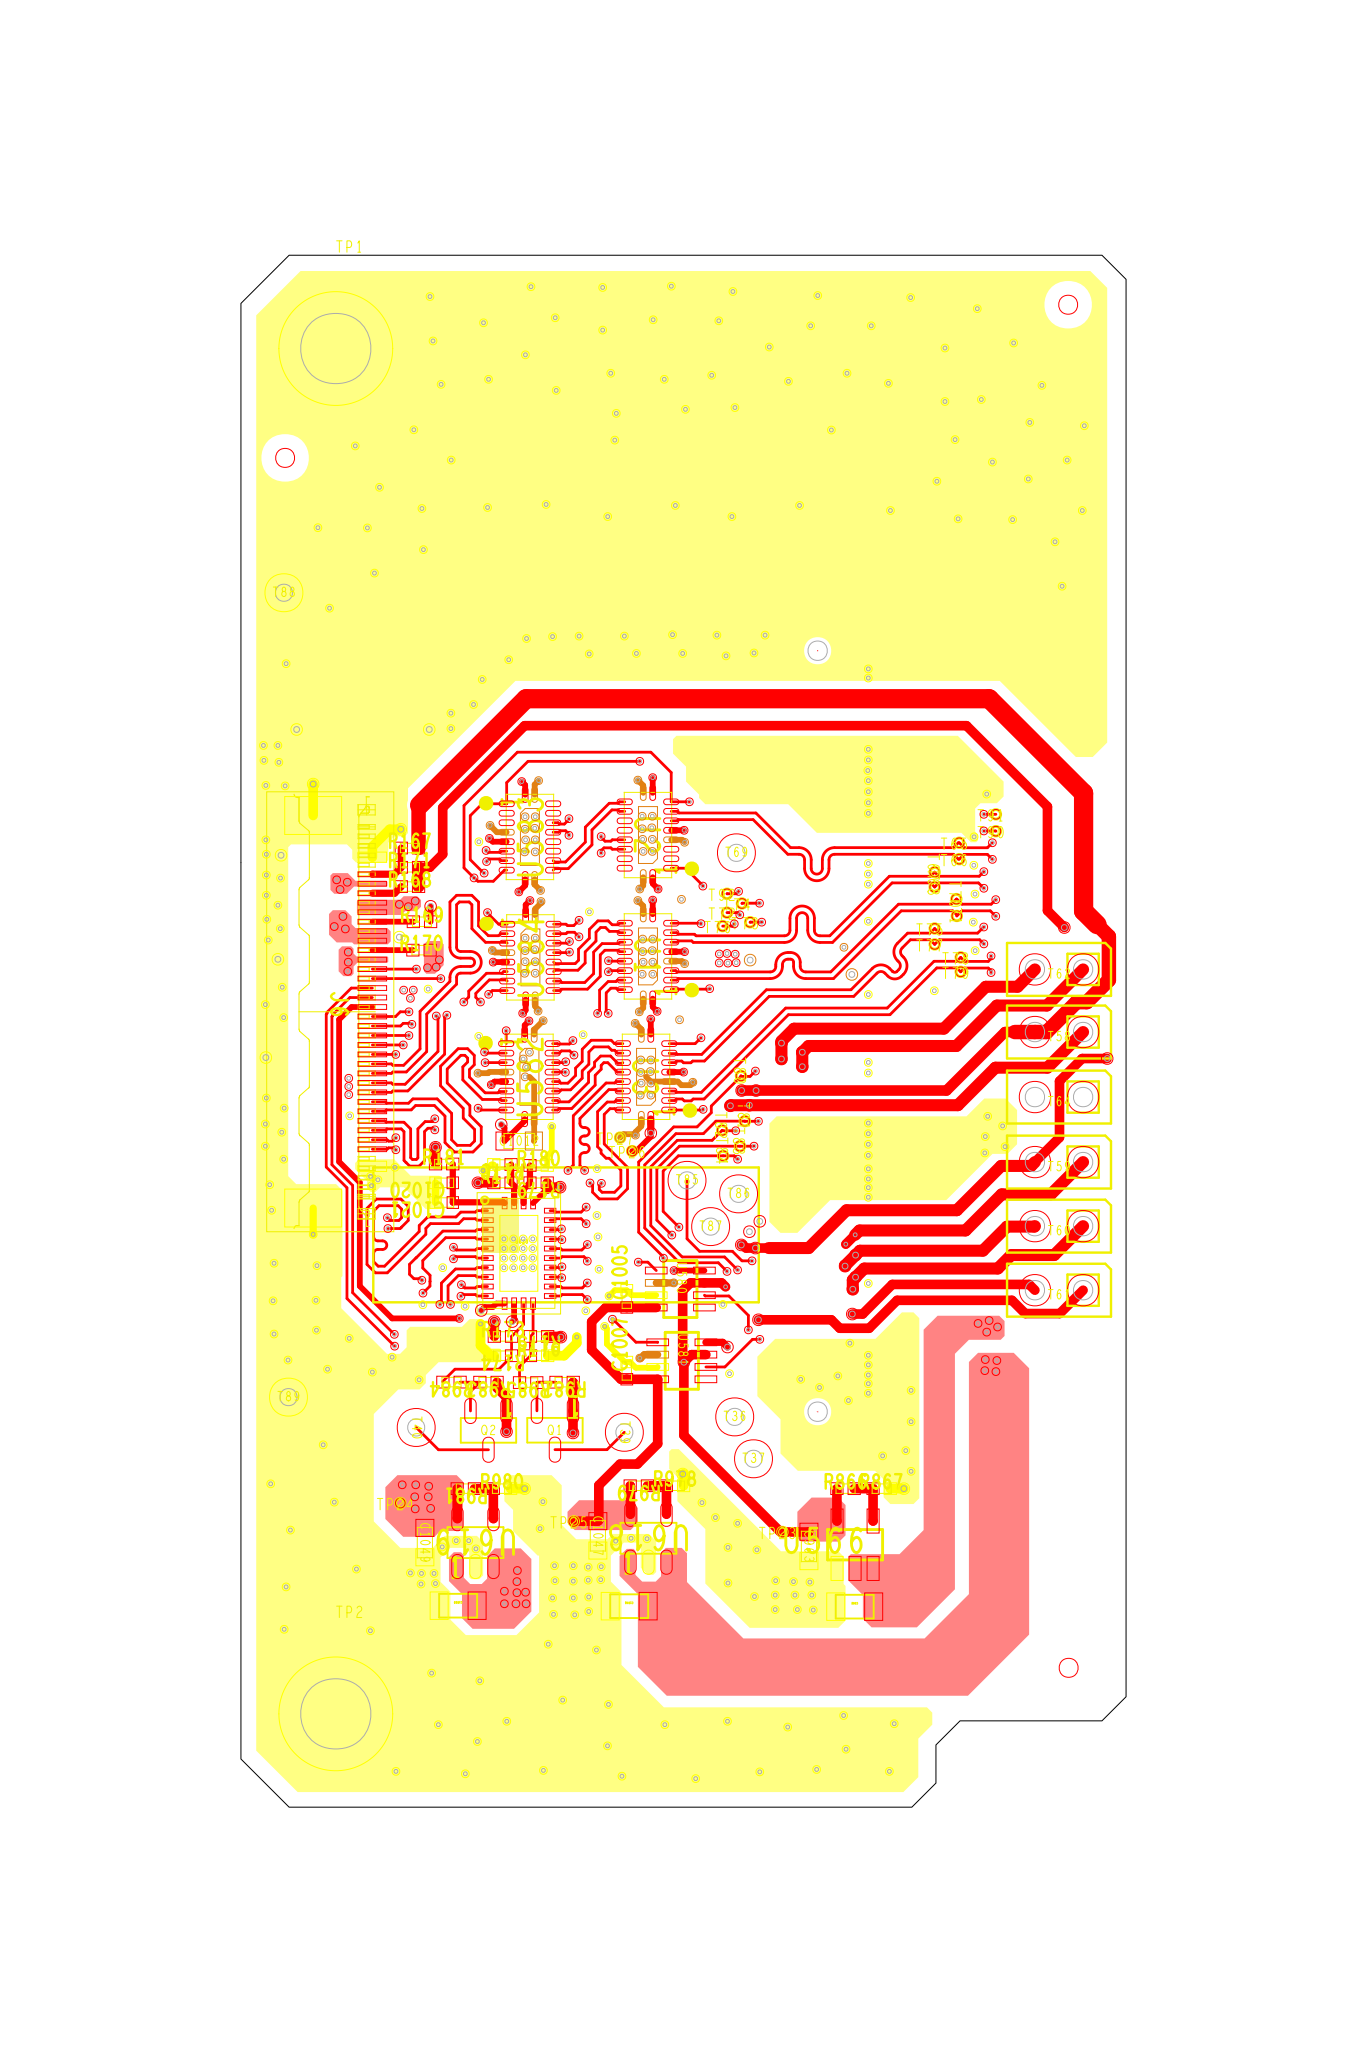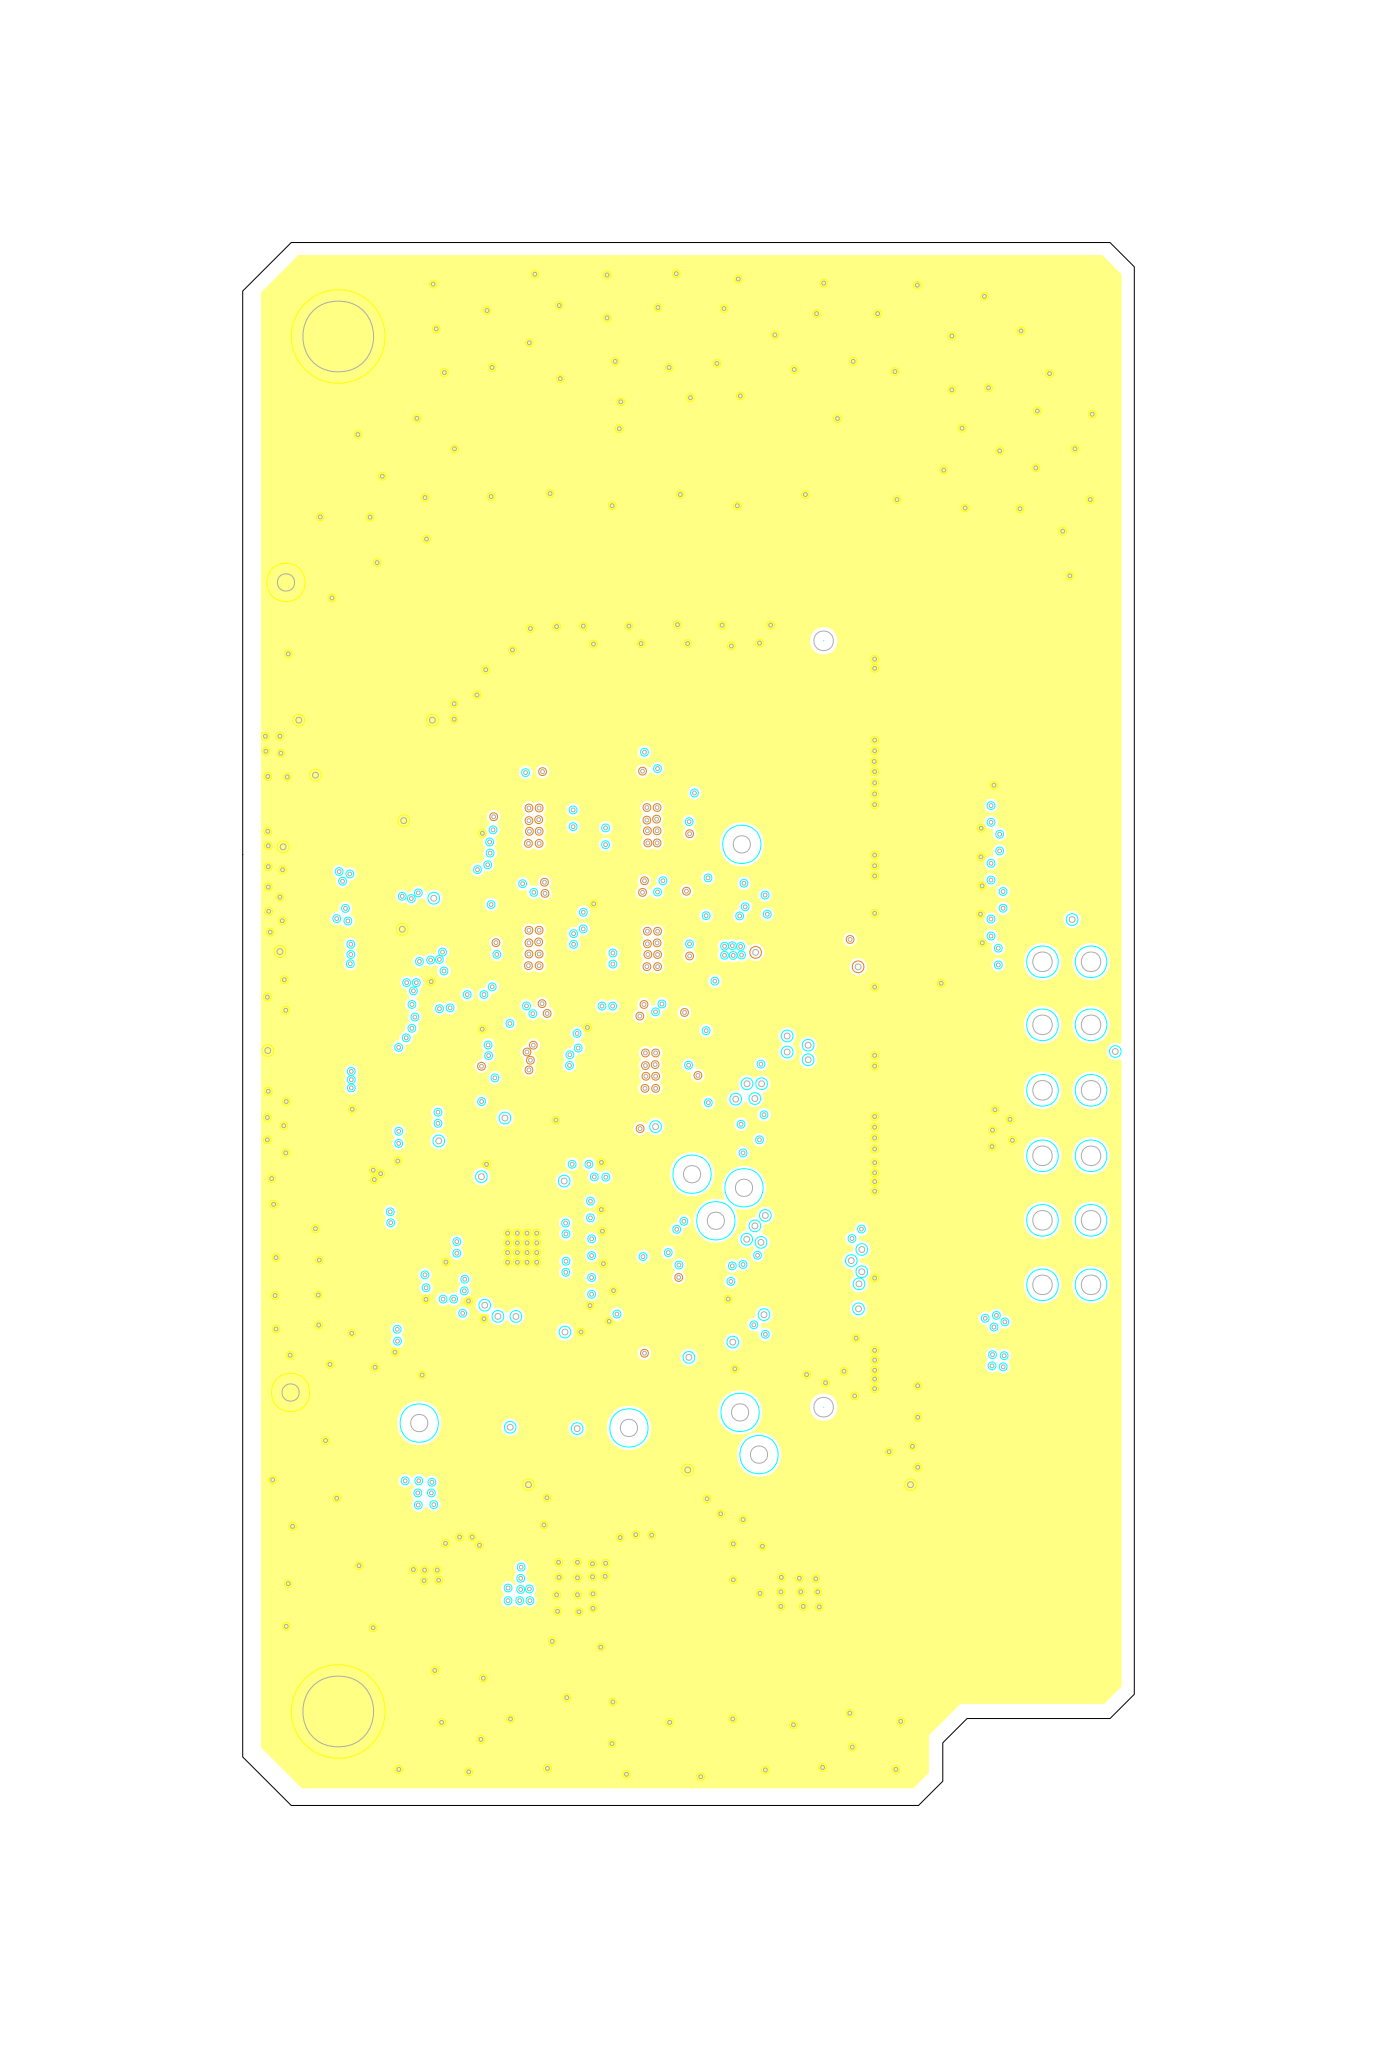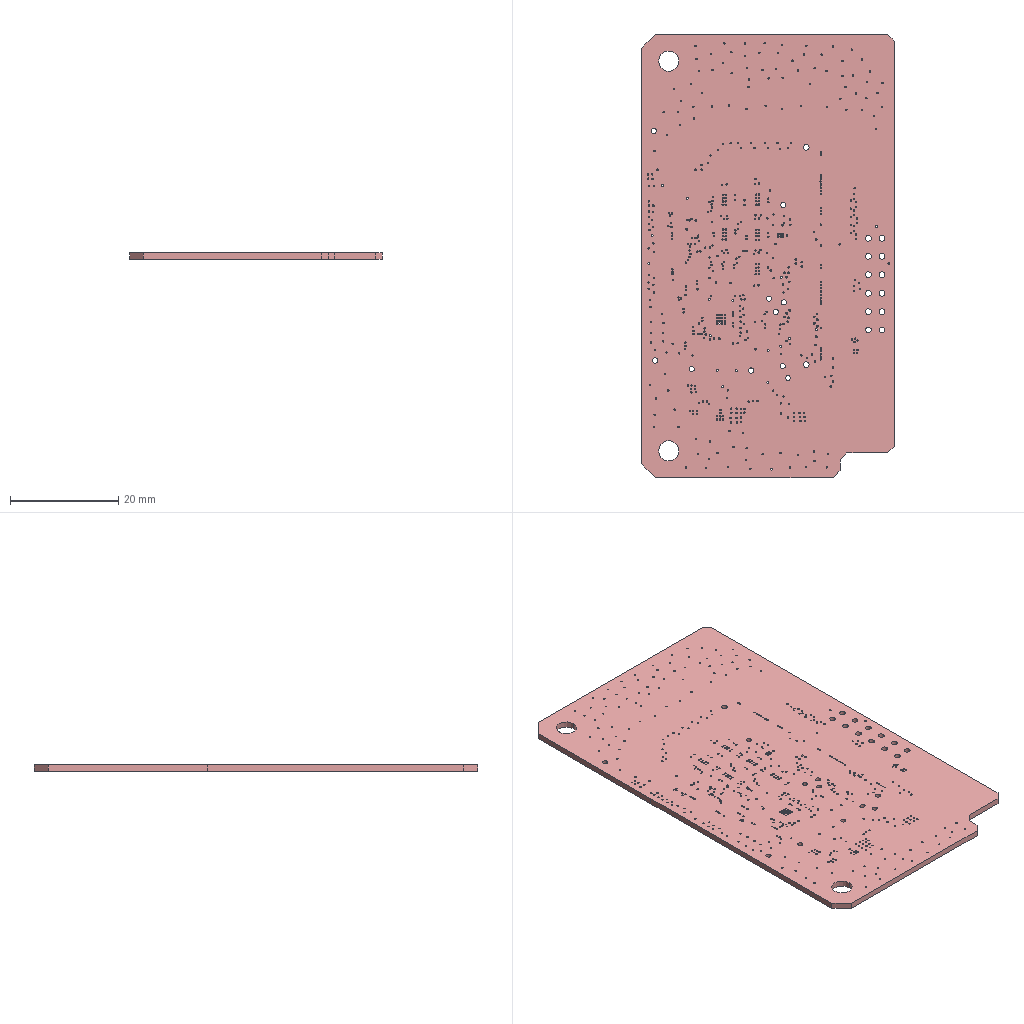Circuit board layout | Cadence Allegro | box 46.7 x 81.8 x 1.1 mm
Layer stack:
# Cadence Allegro layer stack of  (unit mm; from the constraint file cross-section; dielectric type: 0 not recorded (Allegro does not mark core vs prepreg), 3 surface material)
index,name,kind,layer,copper_thickness_mm,dielectric_type,dielectric_thickness_mm,dielectric_material,dielectric_constant
0,Top Surface,other,,,,,,
1,TOP,copper,TOP,0.0305,,,,
2,Dielectric1,dielectric,,,0,0.2032,FR-4,4.5
3,GND2,copper,GND2,0.0305,,,,
4,Dielectric2,dielectric,,,0,0.2032,FR-4,4.5
5,SIG3,copper,SIG3,0.0305,,,,
6,Dielectric3,dielectric,,,0,0.2032,FR-4,4.5
7,SIG4,copper,SIG4,0.0305,,,,
8,Dielectric4,dielectric,,,0,0.2032,FR-4,4.5
9,GND5,copper,GND5,0.0305,,,,
10,Dielectric5,dielectric,,,0,0.2032,FR-4,4.5
11,BOTTOM,copper,BOTTOM,0.0305,,,,
12,Bottom Surface,other,,,,,,
# drill layer pairs: low layer,high layer
drill_pair,TOP,BOTTOM
Part placement:
REFDES,COMP_VALUE,SYM_NAME,SYM_X,SYM_Y,SYM_ROTATE,SYM_MIRROR
C1,10uF,1206C,1040.00,-555.00,0.000,YES
C2,0.1uF,0805C,1050.00,-351.00,0.000,YES
C3,0.1uF,0402C,1790.00,-600.00,90.000,YES
C5,0.1uF,0805C,1220.00,-305.00,180.000,YES
C7,10uF,1206C,1180.00,-540.00,90.000,YES
C9,10uF,1206C,1235.00,70.00,180.000,YES
C10,0.1uF,0805C,1225.00,-135.00,180.000,YES
C13,10uF,1206C,1070.00,70.00,0.000,YES
C14,0.1uF,0805C,1080.00,-135.00,0.000,YES
C667,10nF,0402C,1744.00,-178.00,0.000,YES
C668,10uF,0603C,1744.00,-18.00,0.000,YES
C669,10nF,0402C,1744.00,-435.00,0.000,YES
C670,10uF,0603C,1783.00,-260.00,180.000,YES
C671,10nF,0402C,1740.00,-685.00,0.000,YES
C672,10uF,0603C,1779.00,-507.00,180.000,YES
C962,1uF_12V,0805C,2173.00,-1695.00,180.000,NO
C963,2.2uF,0603C,2078.00,-1570.00,270.000,NO
C1005,0.1uF,0402C,1700.00,-1056.00,90.000,NO
C1006,0.1uF,0402C,1863.00,-1040.00,90.000,YES
C1007,0.1uF,0402C,1700.00,-1205.00,90.000,NO
C1008,0.1uF,0402C,1865.00,-1190.00,90.000,YES
C1009,0.1uF,0402C,1789.00,-103.00,90.000,YES
C1010,0.1uF,0402C,1789.00,-355.00,90.000,YES
C1011,10nF,0402C,1498.00,-505.00,180.000,YES
C1012,10uF,0603C,1476.75,-728.30,0.000,NO
C1013,0.1uF,0402C,1452.74,-572.47,270.000,YES
C1014,0.1uF,0402C,1444.00,-92.00,270.000,YES
C1015,10nF,0402C,1499.00,-12.00,180.000,YES
C1016,10uF,0603C,1494.00,-172.00,180.000,YES
C1017,0.1uF,0402C,1450.00,-337.00,270.000,YES
C1018,10nF,0402C,1500.00,-257.00,180.000,YES
C1019,10uF,0603C,1495.00,-422.00,180.000,YES
C1020,0.1uF,0402C,1321.00,-815.00,180.000,NO
C1021,0.1uF,0402C,1321.00,-856.00,180.000,NO
C1022,0.1uF,0402C,1428.00,-1054.00,270.000,YES
C1023,0.1uF,0402C,1508.00,-1054.00,270.000,YES
C1024,0.01uF,0402C,1468.00,-1054.00,270.000,YES
C1025,0.1uF,0402C,1468.00,-879.00,90.000,YES
C1026,0.01uF,0402C,1508.00,-879.00,90.000,YES
C1047,2.2uF,0603C,1640.00,-1548.00,270.000,NO
C1048,1uF_12V,0805C,1705.00,-1694.00,180.000,NO
C1049,2.2uF,0603C,1281.00,-1562.00,270.000,NO
C1050,1uF_12V,0805C,1350.00,-1693.00,180.000,NO
J2,Z1602,QSH-060-01-X-D-A-MAX,2201.23,-500.28,90.000,YES
J6,CON30,EDP30-0D5-MB,1177.95,-459.93,270.000,NO
LB2,600 ohm,0603L,1090.00,-450.00,270.000,YES
LB3,600 ohm,0603L,1180.00,-405.00,270.000,YES
LB4,600 ohm,0603L,1185.00,-35.00,90.000,YES
LB5,600 ohm,0603L,1120.00,-35.00,90.000,YES
Q1,FDV301N,SOT23_C,1550.95,-1328.77,270.000,NO
Q2,FDV301N,SOT23_C,1413.00,-1329.00,270.000,NO
R167,0R,0402R,1250.00,-120.00,0.000,NO
R168,0R_NC,0402R,1250.00,-200.00,0.000,NO
R169,0R,0402R,1275.00,-273.00,0.000,NO
R170,0R,0402R,1274.00,-332.00,0.000,NO
R171,0R,0402R,1250.00,-160.00,0.000,NO
R172,0R,0402R,1518.56,-1134.53,0.000,YES
R173,4.7k,0402R,1443.00,-1134.00,0.000,NO
R174,10k,0402R,1443.00,-1174.00,180.000,NO
R175,4.7k,0402R,1518.00,-1134.00,180.000,NO
R176,10k,0402R,1518.00,-1174.00,0.000,NO
R177,10k,0402R,1442.00,-815.00,0.000,NO
R178,10k,0402R,1442.00,-777.00,180.000,NO
R179,10k,0402R,1517.00,-815.00,180.000,NO
R180,10k,0402R,1517.00,-779.00,0.000,NO
R181,10k,0402R,1321.00,-776.00,0.000,NO
R866,10k,0402R,2154.00,-1450.00,0.000,NO
R867,5.9k,0402R,2229.00,-1450.00,0.000,NO
R978,6.04k 1%,0402R,1800.00,-1444.00,0.000,NO
R979,10k,0402R,1725.00,-1444.00,180.000,NO
R980,24k 1%,0402R,1441.00,-1450.00,0.000,NO
R981,12.1k,0402R,1366.00,-1450.00,180.000,NO
R982,1k,0402R,1571.00,-1229.00,180.000,NO
R983,1k,0402R,1413.00,-1229.00,180.000,NO
R984,0R,0402R,1336.26,-1228.80,180.000,NO
R985,0R,0402R,1495.36,-1229.80,180.000,NO
T36,T POINT R,TP_C200H90,1924.00,-1301.00,0.000,NO
T37,T POINT R,TP_C200H90,1963.00,-1388.00,0.000,NO
T39,T POINT R,TP_C200H90,1695.00,-1333.00,270.000,NO
T40,T POINT R,TP_C200H90,1263.00,-1323.00,270.000,NO
T58,CON2,CON2_254,2647.00,-502.00,0.000,NO
T59,CON2,CON2_254,2647.00,-772.00,0.000,NO
T60,CON2,CON2_254,2647.00,-905.00,0.000,NO
T61,CON2,CON2_254,2647.00,-1038.00,0.000,NO
T62,CON2,CON2_254,2647.00,-372.00,0.000,NO
T64,CON2,CON2_254,2647.00,-637.00,0.000,NO
T65,T POINT R,TP_C5,2389.99,-109.05,0.000,NO
T66,T POINT R,TP_C5,2389.99,-143.05,0.000,NO
T67,T POINT R,TP_C5,2338.95,-169.99,270.000,NO
T68,T POINT R,TP_C5,2338.95,-200.99,270.000,NO
T69,T POINT R,TP_C200H90,1927.54,-129.96,0.000,NO
T70,T POINT R,TP_C5,2383.95,-225.99,270.000,NO
T71,T POINT R,TP_C5,2384.95,-260.99,270.000,NO
T72,T POINT R,TP_C5,1907.99,-254.05,0.000,NO
T73,T POINT R,TP_C5,1955.99,-274.05,0.000,NO
T74,T POINT R,TP_C5,1938.99,-235.05,0.000,NO
T75,T POINT R,TP_C5,2338.99,-287.05,0.000,NO
T76,T POINT R,TP_C5,1898.99,-282.05,0.000,NO
T77,T POINT R,TP_C5,2338.99,-320.05,0.000,NO
T78,T POINT R,TP_C5,2393.00,-347.00,0.000,NO
T79,T POINT R,TP_C5,2393.00,-377.00,0.000,NO
T80,T POINT R,TP_C5,1937.00,-593.00,270.000,NO
T81,T POINT R,TP_C5,1945.00,-687.00,270.000,NO
T82,T POINT R,TP_C5,1898.00,-706.00,270.000,NO
T83,T POINT R,TP_C5,1935.00,-739.00,270.000,NO
T84,T POINT R,TP_C5,1900.00,-759.00,270.000,NO
T85,T POINT R,TP_C200H90,1825.03,-809.96,0.000,NO
T86,T POINT R,TP_C200H90,1932.03,-837.96,0.000,NO
T87,T POINT R,TP_C200H90,1874.03,-905.96,0.000,NO
T88,T POINT R,TP_C200H90,988.50,410.04,0.000,NO
T89,T POINT R,TP_C200H90,997.99,-1259.96,0.000,NO
T90,T POINT R,TP_C5,2466.00,-85.00,0.000,NO
T91,T POINT R,TP_C5,2466.00,-50.00,0.000,NO
T92,T POINT R,TP_C5,1908.00,-215.00,0.000,NO
TP1,MARK-370-600,MARK-370-600,1096.14,917.05,0.000,NO
TP2,MARK-370-600,MARK-370-600,1096.14,-1917.59,0.000,NO
TP23,T POINT R,TP_C5,2023.00,-1540.00,0.000,NO
TP24,T POINT R,TP_C5,1230.00,-1480.00,0.000,NO
TP25,T POINT R,TP_C5,1590.00,-1518.00,0.000,NO
TP26,T POINT R,TP_C5,1711.09,-749.25,0.000,NO
TP27,T POINT R,TP_C5,1686.09,-721.25,0.000,NO
U1,Z804,VQFN20,1744.00,-345.00,180.000,NO
U2,Z804,VQFN20,1744.00,-93.00,180.000,NO
U3,Z804,VQFN20,1740.00,-595.00,180.000,NO
U566,Z293,UJ_5,2173.79,-1566.46,0.000,NO
U580,Z1578-SPDT,DCN8,1811.18,-1035.60,270.000,NO
U581,Z1578-SPDT,DCN8,1814.18,-1184.58,270.000,NO
U582,Z804,VQFN20,1498.00,-595.00,0.000,NO
U583,Z804,VQFN20,1499.00,-97.00,0.000,NO
U584,Z804,VQFN20,1500.00,-347.00,0.000,NO
U618,Z1023,SOT23_5_C,1745.00,-1553.00,90.000,NO
U619,Z1023,SOT23_5_C,1386.00,-1562.00,90.000,NO
U620,Z2150,WQFN-28,1476.03,-961.48,0.000,NO
Pad and via stacks:
# Allegro (Cadence) via spans and padstacks; design units: ("mils" 2 100)
# via spans: padstack,start_layer,end_layer,net_example,count
VIA12CIR24,ETCH/TOP,ETCH/BOTTOM,GND,47
VIA8CIR16_TB,ETCH/TOP,ETCH/BOTTOM,DC_CSI_GND,1
VIA8CIR16,ETCH/TOP,ETCH/BOTTOM,GND,535
# Allegro padstack definitions: name,start_layer,end_layer,drill,plating,holeType,type
PSM_066X254R,"ETCH/TOP","ETCH/TOP",0.0,"PLATED","none","smd"
PSM_066X470R,"ETCH/TOP","ETCH/TOP",0.0,"PLATED","none","smd"
PSM_030X150R_PM,"ETCH/TOP","ETCH/TOP",0.0,"NON_PLATED","none","smd"
PSM_030X051R,"ETCH/TOP","ETCH/TOP",0.0,"PLATED","none","smd"
PSM_030X070R,"ETCH/TOP","ETCH/TOP",0.0,"PLATED","none","smd"
PSM_040X050,"ETCH/TOP","ETCH/TOP",0.0,"NON_PLATED","none","smd"
PSM_QFN_003X006R_B,"ETCH/TOP","ETCH/TOP",0.0,"PLATED","none","smd"
PSM_QFN_033X005R_NPM,"ETCH/TOP","ETCH/TOP",0.0,"PLATED","none","smd"
PSM_056X061R,"ETCH/TOP","ETCH/TOP",0.0,"PLATED","none","smd"
VST_089C012D,"ETCH/TOP","ETCH/TOP",0.0,"NON_PLATED","none","smd"
PSM_065X041R_NSM,"ETCH/TOP","ETCH/TOP",0.0,"PLATED","none","smd"
PSM_QFN_003X007R_A,"ETCH/TOP","ETCH/TOP",0.0,"PLATED","none","smd"
PSM_160X140R_SM,"ETCH/TOP","ETCH/TOP",0.0,"PLATED","none","smd"
PSM_FID_102_150SM_BOT_TABS,"ETCH/BOTTOM","ETCH/BOTTOM",0.0,"NON_PLATED","none","smd"
PSM_FID_102_150SM_TOP_TABS,"ETCH/TOP","ETCH/TOP",0.0,"NON_PLATED","none","smd"
PSM_FID_130SM,"ETCH/TOP","ETCH/TOP",0.0,"NON_PLATED","none","smd"
PSM_122X112R,"ETCH/TOP","ETCH/TOP",0.0,"NON_PLATED","none","smd"
R028X033S,"ETCH/TOP","ETCH/TOP",0.0,"PLATED","none","smd"
RX19Y2_5,"ETCH/TOP","ETCH/TOP",0.0,"PLATED","none","smd"
R016X050S,"ETCH/TOP","ETCH/TOP",0.0,"PLATED","none","smd"
OX0_40Y1_65T,"ETCH/TOP","ETCH/TOP",0.0,"PLATED","none","smd"
OX0_25Y1_25T,"ETCH/TOP","ETCH/TOP",0.0,"PLATED","none","smd"
RX5_00Y2_00R0_50T,"ETCH/TOP","ETCH/TOP",0.0,"PLATED","none","smd"
REGR2_3R25,"ETCH/TOP","ETCH/TOP",0.0,"PLATED","none","smd"
B160_45,"ETCH/TOP","ETCH/TOP",0.0,"PLATED","none","smd"
R85_95,"ETCH/TOP","ETCH/TOP",0.0,"PLATED","none","smd"
R024X044S,"ETCH/TOP","ETCH/TOP",0.0,"PLATED","none","smd"
PSM_030X150R_PM_20171205,"ETCH/TOP","ETCH/TOP",0.0,"NON_PLATED","none","smd"
REGR017_3R25_20171209,"ETCH/TOP","ETCH/TOP",0.0,"PLATED","none","smd"
VST_071C012D,"ETCH/TOP","ETCH/TOP",0.0,"NON_PLATED","none","smd"
R90_95,"ETCH/TOP","ETCH/TOP",0.0,"PLATED","none","smd"
REGR2_3R25_20171205,"ETCH/TOP","ETCH/TOP",0.0,"PLATED","none","smd"
054150REC,"ETCH/TOP","ETCH/TOP",0.0,"PLATED","none","smd"
025150REC,"ETCH/TOP","ETCH/TOP",0.0,"PLATED","none","smd"
2030REC,"ETCH/TOP","ETCH/TOP",0.0,"PLATED","none","smd"
R64_62,"ETCH/TOP","ETCH/TOP",0.0,"PLATED","none","smd"
SMD0-28_3-5REC,"ETCH/TOP","ETCH/TOP",0.0,"PLATED","none","smd"
SMD2-54_0-43REC,"ETCH/TOP","ETCH/TOP",0.0,"PLATED","none","smd"
SMD4-7_0-43REC,"ETCH/TOP","ETCH/TOP",0.0,"PLATED","none","smd"
R037X067S,"ETCH/TOP","ETCH/TOP",0.0,"PLATED","none","smd"
R95_145,"ETCH/TOP","ETCH/TOP",0.0,"PLATED","none","smd"
R030X035S,"ETCH/TOP","ETCH/TOP",0.0,"PLATED","none","smd"
C5,"ETCH/TOP","ETCH/TOP",0.0,"PLATED","none","smd"
R60_62,"ETCH/TOP","ETCH/TOP",0.0,"PLATED","none","smd"
B132_60,"ETCH/TOP","ETCH/TOP",0.0,"PLATED","none","smd"
B80_30,"ETCH/TOP","ETCH/TOP",0.0,"PLATED","none","smd"
R100_300C10,"ETCH/TOP","ETCH/TOP",0.0,"PLATED","none","smd"
SMD25_50,"ETCH/TOP","ETCH/TOP",0.0,"PLATED","none","smd"
SMD14_45,"ETCH/TOP","ETCH/TOP",0.0,"PLATED","none","smd"
B127_60,"ETCH/TOP","ETCH/TOP",0.0,"PLATED","none","smd"
REC_2X4,"ETCH/TOP","ETCH/TOP",0.0,"NON_PLATED","none","smd"
REC_0-25X0-6,"ETCH/TOP","ETCH/TOP",0.0,"PLATED","none","smd"
MARK_C1R00_C2R30NP,"ETCH/TOP","ETCH/TOP",0.0,"PLATED","none","smd"
NTH_109P,"ETCH/TOP","ETCH/BOTTOM",42.91,"NON_PLATED","circle_drill","through"
PTH_599C_INT422C_B701C320P,"ETCH/TOP","ETCH/BOTTOM",125.98,"PLATED","circle_drill","through"
VTH_048C028P,"ETCH/TOP","ETCH/BOTTOM",11.02,"PLATED","circle_drill","through"
NTH_300P_TOOLINGHOLE,"ETCH/TOP","ETCH/BOTTOM",118.11,"NON_PLATED","circle_drill","through"
NTH_050P,"ETCH/TOP","ETCH/BOTTOM",19.69,"NON_PLATED","circle_drill","through"
PAD1_70D0_90,"ETCH/TOP","ETCH/BOTTOM",35.43,"PLATED","circle_drill","through"
PAD1_70D0_90S,"ETCH/TOP","ETCH/BOTTOM",35.43,"PLATED","circle_drill","through"
VIA8CIR16,"ETCH/TOP","ETCH/BOTTOM",8.0,"PLATED","circle_drill","through"
VIA8CIR16_TB,"ETCH/TOP","ETCH/BOTTOM",7.99,"PLATED","circle_drill","through"
VIA12CIR24_TB,"ETCH/TOP","ETCH/BOTTOM",12.01,"PLATED","circle_drill","through"
VIA12CIR24,"ETCH/TOP","ETCH/BOTTOM",12.01,"PLATED","circle_drill","through"
VIA8CIR16_TOP,"ETCH/TOP","ETCH/BOTTOM",7.99,"PLATED","circle_drill","through"
PAD_MTG430_650,"ETCH/TOP","ETCH/BOTTOM",169.29,"PLATED","circle_drill","through"
C170H90,"ETCH/TOP","ETCH/BOTTOM",35.43,"PLATED","circle_drill","through"
S170H90,"ETCH/TOP","ETCH/BOTTOM",35.43,"PLATED","circle_drill","through"
C200H90,"ETCH/TOP","ETCH/BOTTOM",35.43,"PLATED","circle_drill","through"
NPTH1-02CIR,"ETCH/TOP","ETCH/BOTTOM",40.16,"NON_PLATED","circle_drill","through"
PTH_165C102P,"ETCH/TOP","ETCH/BOTTOM",40.16,"PLATED","circle_drill","through"
PAD_MTG370_600,"ETCH/TOP","ETCH/BOTTOM",145.67,"PLATED","circle_drill","through"
V_C60H30,"ETCH/TOP","ETCH/BOTTOM",11.81,"PLATED","circle_drill","through"
Design rules, without the lines most boards share, first 16 of 62 lines:
# Cadence Allegro design rules of  (from the Constraint Manager export constraints.dcfx, design unit mil; typed fields in mm)
# columns: name | kind | enabled | priority | scope1 | scope2 | descriptor | typed fields (field=value)
# Allegro precedence (priority 1 wins): 1 Region class-to-class, 2 Region class, 3 Region, 4 class-to-class, 5 DiffPair/Bus/NetGroup override, 6 NetClass, 7 constraint set (CSet) default
# per-layer values are written LAYER=value in the descriptor and LAYER:mm in the typed field; a maximum of 0 means no limit set
# --- net classes (and buses / net groups) ---
BUFF_OUT | NetClass | enabled | 6 | BUFF_CLKN_TR1C_OUT, BUFF_CLKP_TR0C_OUT, BUFF_D0N_TR0B_OUT, BUFF_D0P_TR0A_OUT, BUFF_D1N_TR1B_OUT, BUFF_D1P_TR1A_OUT, BUFF_D2N_TR2B_OUT, BUFF_D2P_TR2A_OUT, BUFF_D3N_NC_OUT, BUFF_D3P_NC_OUT | All | Net Class (members: 10 Net) |
BUFF_IN | NetClass | enabled | 6 | BUFF_CLK_IN, BUFF_D0_IN, BUFF_D1_IN, BUFF_D2_IN, BUFF_D3_IN | All | Net Class (members: 5 DiffPair) |
OS_MIPI | NetClass | enabled | 6 | OS_MIPI_CLKN, OS_MIPI_CLKP, OS_MIPI_D0N, OS_MIPI_D0P, OS_MIPI_D1N, OS_MIPI_D1P, OS_MIPI_D2N, OS_MIPI_D2P, OS_MIPI_D3N, OS_MIPI_D3P | All | Net Class (members: 10 Net) |
CSI | NetClass | enabled | 6 | CSI_CLK, CSI_D0_TR0, CSI_D1, CSI_D2, CSI_D3 | All | Net Class (members: 5 DiffPair) |
OX | NetClass | enabled | 6 | OX_CLKN, OX_CLKP, OX_D0N, OX_D0P, OX_D1N, OX_D1P, OX_D2N, OX_D2P, OX_D3N, OX_D3P | All | Net Class (members: 10 Net) |
# --- track widths, neck and differential-pair gap (physical constraint sets) ---
95OHM_DIFF_JLC2313_6L | PhysicalCSet | enabled | 7 | DiffPair(24): BUFF_CLK_IN, BUFF_D0_IN, BUFF_D1_IN, BUFF_D2_IN, BUFF_D3_IN, CSI_CLK, CSI_D0_TR0, CSI_D1, CSI_D2, CSI_D3, OX_D3, OX_D2, ... | All | Physical Constraint (Min Line Width=5.78mil) (Max Line Width=5.78mil) (Min Neck Width=4mil) (Max Neck Length=5000mil) (DiffPair Primary Gap=8mil) (DiffPair Neck Gap=4mil) (DiffPair Min Space=4mil) (DiffPair Coupled +Tol=0mil) (DiffPair Coupled -Tol=0mil) (Min BB Via Stagger=5mil) (Max BB Via Stagger=0mil) (T-junctions=ANYWHERE) (Pad-pad direct connect=ALL_ALLOWED) (Allowed vias=VIA8CIR16, VIA12CIR24, VIA8CIR16_TB, VIA12CIR24_TB, VIA8CIR16_TOP) | min_line_width=0.1468 min_neck_width=0.1016 min_bvia_stagger=0.127 max_bvia_stagger=0 ts_allowed=ANYWHERE diffp_primary_gap=0.2032 diffp_neck_gap=0.1016 max_line_width=0.1468 maximum_neck_length=127 pad_pad_direct_connect=ALL_ALLOWED allow_on_etch_subclass=TRUE diffp_coupled_plus=0 diffp_coupled_minus=0 diffp_min_space=0.1016 vias=VIA8CIR16,VIA12CIR24,VIA8CIR16_TB,VIA12CIR24_TB,VIA8CIR16_TOP
50OHM_SIG_JCL2313 | PhysicalCSet | enabled | 7 | not referenced | All | Physical Constraint (Min Line Width=5.78mil) (Max Line Width=TOP=6mil GND2=6mil SIG3=5.78mil SIG4=6mil GND5=6mil BOTTOM=6mil) (Min Neck Width=5.78mil) (Max Neck Length=5.78mil) (DiffPair Primary Gap=6.78mil) (DiffPair Neck Gap=6.78mil) (DiffPair Min Space=6.78mil) (DiffPair Coupled +Tol=6.78mil) (DiffPair Coupled -Tol=6.78mil) (Min BB Via Stagger=6.78mil) (Max BB Via Stagger=6.78mil) (T-junctions=ANYWHERE) (Pad-pad direct connect=ALL_ALLOWED) (Allowed vias=VIA8CIR16, VIA8CIR16_TB, VIA12CIR24_TB, VIA12CIR24, VIA8CIR16_TOP) | min_line_width=0.1468 min_neck_width=0.1468 min_bvia_stagger=0.1722 max_bvia_stagger=0.1722 ts_allowed=ANYWHERE diffp_primary_gap=0.1722 diffp_neck_gap=0.1722 max_line_width=TOP:0.1524,GND2:0.1524,SIG3:0.1468,SIG4:0.1524,GND5:0.1524,BOTTOM:0.1524 maximum_neck_length=0.1468 pad_pad_direct_connect=ALL_ALLOWED allow_on_etch_subclass=TRUE diffp_coupled_plus=0.1722 diffp_coupled_minus=0.1722 diffp_min_space=0.1722 vias=VIA8CIR16,VIA8CIR16_TB,VIA12CIR24_TB,VIA12CIR24,VIA8CIR16_TOP
100_OHM_DIFF | PhysicalCSet | enabled | 7 | not referenced | All | Physical Constraint (Min Line Width=6mil) (Max Line Width=6mil) (Min Neck Width=4mil) (Max Neck Length=100mil) (DiffPair Primary Gap=6mil) (DiffPair Neck Gap=0mil) (DiffPair Min Space=6mil) (DiffPair Coupled +Tol=0mil) (DiffPair Coupled -Tol=0mil) (Min BB Via Stagger=5mil) (Max BB Via Stagger=0mil) (T-junctions=ANYWHERE) (Pad-pad direct connect=ALL_ALLOWED) (Allowed vias=VIA8CIR16, VIA8CIR16_TB, VIA12CIR24_TB, VIA12CIR24, VIA8CIR16_TOP) | min_line_width=0.1524 min_neck_width=0.1016 min_bvia_stagger=0.127 max_bvia_stagger=0 ts_allowed=ANYWHERE diffp_primary_gap=0.1524 diffp_neck_gap=0 max_line_width=0.1524 maximum_neck_length=2.54 pad_pad_direct_connect=ALL_ALLOWED allow_on_etch_subclass=TRUE diffp_coupled_plus=0 diffp_coupled_minus=0 diffp_min_space=0.1524 vias=VIA8CIR16,VIA8CIR16_TB,VIA12CIR24_TB,VIA12CIR24,VIA8CIR16_TOP
DEFAULT | PhysicalCSet | enabled | 7 | Design default; Region(1): USB_HUB | All | Physical Constraint (Min Line Width=6mil) (Max Line Width=0mil) (Min Neck Width=4mil) (Max Neck Length=5000mil) (DiffPair Primary Gap=0mil) (DiffPair Neck Gap=0mil) (DiffPair Min Space=0mil) (DiffPair Coupled +Tol=0mil) (DiffPair Coupled -Tol=0mil) (Min BB Via Stagger=5mil) (Max BB Via Stagger=0mil) (T-junctions=ANYWHERE) (Pad-pad direct connect=ALL_ALLOWED) (Allowed vias=VIA8CIR16, VIA12CIR24, VIA8CIR16_TB, VIA12CIR24_TB, VIA8CIR16_TOP) | min_line_width=0.1524 min_neck_width=0.1016 min_bvia_stagger=0.127 max_bvia_stagger=0 ts_allowed=ANYWHERE diffp_primary_gap=0 diffp_neck_gap=0 max_line_width=0 maximum_neck_length=127 pad_pad_direct_connect=ALL_ALLOWED allow_on_etch_subclass=TRUE diffp_coupled_plus=0 diffp_coupled_minus=0 diffp_min_space=0 vias=VIA8CIR16,VIA12CIR24,VIA8CIR16_TB,VIA12CIR24_TB,VIA8CIR16_TOP
# --- clearances: line / pad / via / shape / hole (spacing constraint sets) ---